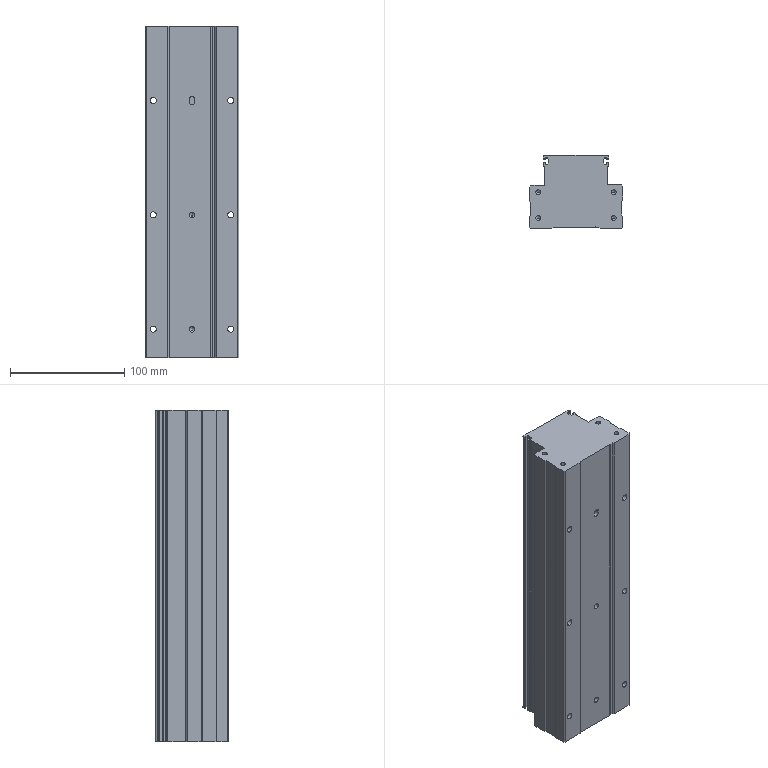Part | STEP file | 1 solid | 119 faces | box 82 x 64 x 290 mm | volume 1277181 mm3 | plane 62 | cylinder 45 | cone 12 | commonest cylinder face diameters 0.6 x12 5.4 x12 4.2 x8 5 x6 2 x5 3 x2